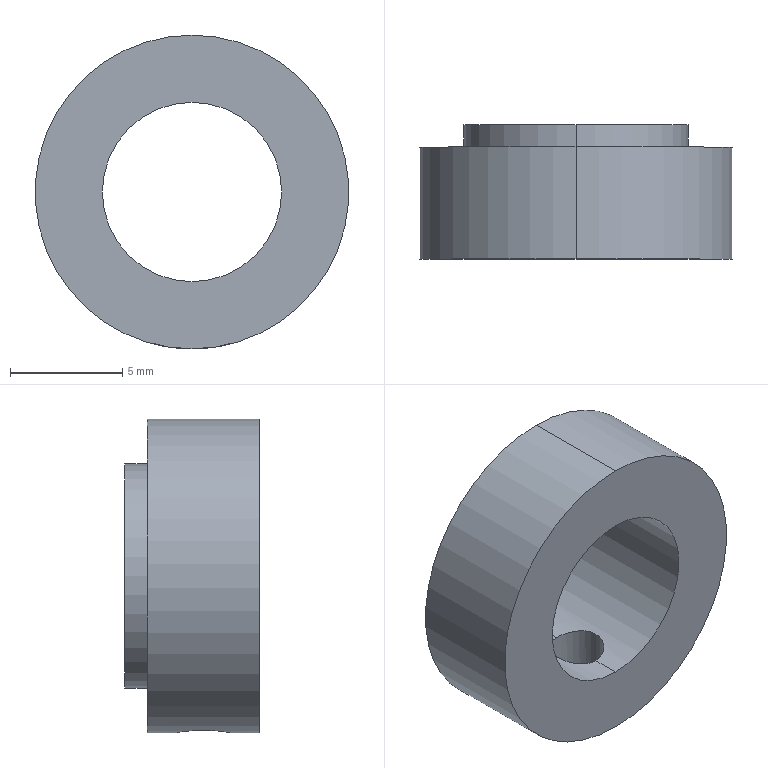Part | SolidWorks | features ICE 1, Revolution 1 | 1 solid | 11 faces | box 14 x 6 x 14 mm | volume 531.806 mm3 | cylinder 8 | plane 3 | commonest cylinder face diameters 2.5 x2 8 x2 10 x2 14 x2
STEP:
#1=CARTESIAN_POINT('',(0.,-0.3817,-7.));
#2=VERTEX_POINT('',#1);
#3=CARTESIAN_POINT('',(-1.25,0.8683,-6.887));
#4=VERTEX_POINT('',#3);
#5=CARTESIAN_POINT('',(0.,-0.3817,-7.));
#6=CARTESIAN_POINT('',(-0.1634,-0.3817,-7.));
#7=CARTESIAN_POINT('',(-0.3282,-0.3488,-6.994));
#8=CARTESIAN_POINT('',(-0.6292,-0.224,-6.973));
#9=CARTESIAN_POINT('',(-0.7683,-0.1311,-6.959));
#10=CARTESIAN_POINT('',(-0.9412,0.04171,-6.937));
#11=CARTESIAN_POINT('',(-0.994,0.1059,-6.929));
#12=CARTESIAN_POINT('',(-1.085,0.2414,-6.916));
#13=CARTESIAN_POINT('',(-1.123,0.3131,-6.909));
#14=CARTESIAN_POINT('',(-1.217,0.5406,-6.894));
#15=CARTESIAN_POINT('',(-1.25,0.7031,-6.887));
#16=CARTESIAN_POINT('',(-1.25,0.8683,-6.887));
#17=B_SPLINE_CURVE_WITH_KNOTS('',3,(#5,#6,#7,#8,#9,#10,#11,#12,#13,#14,#15,#16),.UNSPECIFIED.,.F.,.F.,(4,2,2,2,2,4),(0.003916,0.004405,0.004895,0.00514,0.005385,0.005874),.UNSPECIFIED.);
#18=EDGE_CURVE('',#2,#4,#17,.T.);
#19=ORIENTED_EDGE('',*,*,#18,.T.);
#20=CARTESIAN_POINT('',(-1.25,0.8683,-3.8));
#21=VERTEX_POINT('',#20);
#22=CARTESIAN_POINT('',(-1.25,0.8683,-10.));
#23=DIRECTION('',(0.,0.,1.));
#24=VECTOR('',#23,1000.);
#25=LINE('',#22,#24);
#26=EDGE_CURVE('',#4,#21,#25,.T.);
#27=ORIENTED_EDGE('',*,*,#26,.T.);
#28=CARTESIAN_POINT('',(0.,-0.3817,-4.));
#29=VERTEX_POINT('',#28);
#30=CARTESIAN_POINT('',(-1.25,0.8683,-3.8));
#31=CARTESIAN_POINT('',(-1.25,0.7862,-3.8));
#32=CARTESIAN_POINT('',(-1.242,0.7028,-3.802));
#33=CARTESIAN_POINT('',(-1.209,0.5421,-3.813));
#34=CARTESIAN_POINT('',(-1.186,0.4639,-3.82));
#35=CARTESIAN_POINT('',(-1.091,0.236,-3.849));
#36=CARTESIAN_POINT('',(-0.9987,0.09902,-3.875));
#37=CARTESIAN_POINT('',(-0.8257,-0.0737,-3.914));
#38=CARTESIAN_POINT('',(-0.7632,-0.125,-3.927));
#39=CARTESIAN_POINT('',(-0.6281,-0.2155,-3.951));
#40=CARTESIAN_POINT('',(-0.5549,-0.2548,-3.962));
#41=CARTESIAN_POINT('',(-0.329,-0.3486,-3.989));
#42=CARTESIAN_POINT('',(-0.1638,-0.3817,-4.));
#43=CARTESIAN_POINT('',(0.,-0.3817,-4.));
#44=B_SPLINE_CURVE_WITH_KNOTS('',3,(#30,#31,#32,#33,#34,#35,#36,#37,#38,#39,#40,#41,#42,#43),.UNSPECIFIED.,.F.,.F.,(4,2,2,2,2,2,4),(0.001967,0.002213,0.002458,0.00295,0.003196,0.003441,0.003933),.UNSPECIFIED.);
#45=EDGE_CURVE('',#21,#29,#44,.T.);
#46=ORIENTED_EDGE('',*,*,#45,.T.);
#47=CARTESIAN_POINT('',(1.25,0.8683,-3.8));
#48=VERTEX_POINT('',#47);
#49=CARTESIAN_POINT('',(0.,-0.3817,-4.));
#50=CARTESIAN_POINT('',(0.1638,-0.3817,-4.));
#51=CARTESIAN_POINT('',(0.3292,-0.3486,-3.989));
#52=CARTESIAN_POINT('',(0.6307,-0.2232,-3.953));
#53=CARTESIAN_POINT('',(0.7685,-0.131,-3.927));
#54=CARTESIAN_POINT('',(0.9992,0.09974,-3.875));
#55=CARTESIAN_POINT('',(1.091,0.236,-3.849));
#56=CARTESIAN_POINT('',(1.186,0.4643,-3.82));
#57=CARTESIAN_POINT('',(1.21,0.5424,-3.813));
#58=CARTESIAN_POINT('',(1.242,0.7027,-3.802));
#59=CARTESIAN_POINT('',(1.25,0.7859,-3.8));
#60=CARTESIAN_POINT('',(1.25,0.8683,-3.8));
#61=B_SPLINE_CURVE_WITH_KNOTS('',3,(#49,#50,#51,#52,#53,#54,#55,#56,#57,#58,#59,#60),.UNSPECIFIED.,.F.,.F.,(4,2,2,2,2,4),(0.003933,0.004424,0.004916,0.005407,0.005653,0.005899),.UNSPECIFIED.);
#62=EDGE_CURVE('',#29,#48,#61,.T.);
#63=ORIENTED_EDGE('',*,*,#62,.T.);
#64=CARTESIAN_POINT('',(1.25,0.8683,-6.887));
#65=VERTEX_POINT('',#64);
#66=CARTESIAN_POINT('',(1.25,0.8683,-10.));
#67=DIRECTION('',(0.,0.,1.));
#68=VECTOR('',#67,1000.);
#69=LINE('',#66,#68);
#70=EDGE_CURVE('',#65,#48,#69,.T.);
#71=ORIENTED_EDGE('',*,*,#70,.F.);
#72=CARTESIAN_POINT('',(1.25,0.8683,-6.887));
#73=CARTESIAN_POINT('',(1.25,0.7866,-6.887));
#74=CARTESIAN_POINT('',(1.242,0.7036,-6.889));
#75=CARTESIAN_POINT('',(1.21,0.5432,-6.895));
#76=CARTESIAN_POINT('',(1.186,0.4652,-6.899));
#77=CARTESIAN_POINT('',(1.092,0.238,-6.915));
#78=CARTESIAN_POINT('',(1.,0.1005,-6.929));
#79=CARTESIAN_POINT('',(0.7674,-0.1321,-6.959));
#80=CARTESIAN_POINT('',(0.6298,-0.2238,-6.973));
#81=CARTESIAN_POINT('',(0.3275,-0.3491,-6.994));
#82=CARTESIAN_POINT('',(0.1633,-0.3817,-7.));
#83=CARTESIAN_POINT('',(0.,-0.3817,-7.));
#84=B_SPLINE_CURVE_WITH_KNOTS('',3,(#72,#73,#74,#75,#76,#77,#78,#79,#80,#81,#82,#83),.UNSPECIFIED.,.F.,.F.,(4,2,2,2,2,4),(0.001958,0.002203,0.002448,0.002937,0.003427,0.003916),.UNSPECIFIED.);
#85=EDGE_CURVE('',#65,#2,#84,.T.);
#86=ORIENTED_EDGE('',*,*,#85,.T.);
#87=EDGE_LOOP('',(#19,#27,#46,#63,#71,#86));
#88=FACE_OUTER_BOUND('',#87,.T.);
#89=CARTESIAN_POINT('',(0.,0.8683,-10.));
#90=DIRECTION('',(0.,0.,1.));
#91=DIRECTION('',(1.,0.,0.));
#92=AXIS2_PLACEMENT_3D('',#89,#90,#91);
#93=CYLINDRICAL_SURFACE('',#92,1.25);
#94=ADVANCED_FACE('',(#88),#93,.F.);
#95=CARTESIAN_POINT('',(0.,3.368,-7.));
#96=VERTEX_POINT('',#95);
#97=CARTESIAN_POINT('',(0.,3.368,7.));
#98=VERTEX_POINT('',#97);
#99=CARTESIAN_POINT('',(0.,3.368,0.));
#100=DIRECTION('',(0.,-1.,0.));
#101=DIRECTION('',(0.,0.,-1.));
#102=AXIS2_PLACEMENT_3D('',#99,#100,#101);
#103=CIRCLE('',#102,7.);
#104=EDGE_CURVE('',#96,#98,#103,.T.);
#105=ORIENTED_EDGE('',*,*,#104,.T.);
#106=CARTESIAN_POINT('',(0.,-1.632,7.));
#107=VERTEX_POINT('',#106);
#108=CARTESIAN_POINT('',(0.,0.,7.));
#109=DIRECTION('',(0.,-1.,0.));
#110=VECTOR('',#109,1000.);
#111=LINE('',#108,#110);
#112=EDGE_CURVE('',#98,#107,#111,.T.);
#113=ORIENTED_EDGE('',*,*,#112,.T.);
#114=CARTESIAN_POINT('',(0.,-1.632,-7.));
#115=VERTEX_POINT('',#114);
#116=CARTESIAN_POINT('',(0.,-1.632,0.));
#117=DIRECTION('',(0.,-1.,0.));
#118=DIRECTION('',(0.,0.,-1.));
#119=AXIS2_PLACEMENT_3D('',#116,#117,#118);
#120=CIRCLE('',#119,7.);
#121=EDGE_CURVE('',#115,#107,#120,.T.);
#122=ORIENTED_EDGE('',*,*,#121,.F.);
#123=CARTESIAN_POINT('',(0.,0.,-7.));
#124=DIRECTION('',(0.,-1.,0.));
#125=VECTOR('',#124,1000.);
#126=LINE('',#123,#125);
#127=EDGE_CURVE('',#2,#115,#126,.T.);
#128=ORIENTED_EDGE('',*,*,#127,.F.);
#129=ORIENTED_EDGE('',*,*,#85,.F.);
#130=CARTESIAN_POINT('',(0.,2.118,-7.));
#131=VERTEX_POINT('',#130);
#132=CARTESIAN_POINT('',(0.,2.118,-7.));
#133=CARTESIAN_POINT('',(0.1656,2.118,-7.));
#134=CARTESIAN_POINT('',(0.328,2.086,-6.994));
#135=CARTESIAN_POINT('',(0.6307,1.96,-6.973));
#136=CARTESIAN_POINT('',(0.7692,1.867,-6.959));
#137=CARTESIAN_POINT('',(0.9993,1.637,-6.929));
#138=CARTESIAN_POINT('',(1.092,1.497,-6.915));
#139=CARTESIAN_POINT('',(1.217,1.197,-6.894));
#140=CARTESIAN_POINT('',(1.25,1.032,-6.887));
#141=CARTESIAN_POINT('',(1.25,0.8683,-6.887));
#142=B_SPLINE_CURVE_WITH_KNOTS('',3,(#132,#133,#134,#135,#136,#137,#138,#139,#140,#141),.UNSPECIFIED.,.F.,.F.,(4,2,2,2,4),(0.,0.0004896,0.0009792,0.001469,0.001958),.UNSPECIFIED.);
#143=EDGE_CURVE('',#131,#65,#142,.T.);
#144=ORIENTED_EDGE('',*,*,#143,.F.);
#145=CARTESIAN_POINT('',(0.,0.,-7.));
#146=DIRECTION('',(0.,-1.,0.));
#147=VECTOR('',#146,1000.);
#148=LINE('',#145,#147);
#149=EDGE_CURVE('',#96,#131,#148,.T.);
#150=ORIENTED_EDGE('',*,*,#149,.F.);
#151=EDGE_LOOP('',(#105,#113,#122,#128,#129,#144,#150));
#152=FACE_OUTER_BOUND('',#151,.T.);
#153=CARTESIAN_POINT('',(0.,0.,0.));
#154=DIRECTION('',(0.,-1.,0.));
#155=DIRECTION('',(0.,0.,-1.));
#156=AXIS2_PLACEMENT_3D('',#153,#154,#155);
#157=CYLINDRICAL_SURFACE('',#156,7.);
#158=ADVANCED_FACE('',(#152),#157,.T.);
#159=CARTESIAN_POINT('',(0.,4.368,-5.));
#160=VERTEX_POINT('',#159);
#161=CARTESIAN_POINT('',(0.,4.368,5.));
#162=VERTEX_POINT('',#161);
#163=CARTESIAN_POINT('',(0.,4.368,0.));
#164=DIRECTION('',(0.,-1.,0.));
#165=DIRECTION('',(0.,0.,-1.));
#166=AXIS2_PLACEMENT_3D('',#163,#164,#165);
#167=CIRCLE('',#166,5.);
#168=EDGE_CURVE('',#160,#162,#167,.T.);
#169=ORIENTED_EDGE('',*,*,#168,.T.);
#170=CARTESIAN_POINT('',(0.,3.368,5.));
#171=VERTEX_POINT('',#170);
#172=CARTESIAN_POINT('',(0.,0.,5.));
#173=DIRECTION('',(0.,-1.,0.));
#174=VECTOR('',#173,1000.);
#175=LINE('',#172,#174);
#176=EDGE_CURVE('',#162,#171,#175,.T.);
#177=ORIENTED_EDGE('',*,*,#176,.T.);
#178=CARTESIAN_POINT('',(0.,3.368,-5.));
#179=VERTEX_POINT('',#178);
#180=CARTESIAN_POINT('',(0.,3.368,0.));
#181=DIRECTION('',(0.,-1.,0.));
#182=DIRECTION('',(0.,0.,-1.));
#183=AXIS2_PLACEMENT_3D('',#180,#181,#182);
#184=CIRCLE('',#183,5.);
#185=EDGE_CURVE('',#179,#171,#184,.T.);
#186=ORIENTED_EDGE('',*,*,#185,.F.);
#187=CARTESIAN_POINT('',(0.,0.,-5.));
#188=DIRECTION('',(0.,-1.,0.));
#189=VECTOR('',#188,1000.);
#190=LINE('',#187,#189);
#191=EDGE_CURVE('',#160,#179,#190,.T.);
#192=ORIENTED_EDGE('',*,*,#191,.F.);
#193=EDGE_LOOP('',(#169,#177,#186,#192));
#194=FACE_OUTER_BOUND('',#193,.T.);
#195=CARTESIAN_POINT('',(0.,0.,0.));
#196=DIRECTION('',(0.,-1.,0.));
#197=DIRECTION('',(0.,0.,-1.));
#198=AXIS2_PLACEMENT_3D('',#195,#196,#197);
#199=CYLINDRICAL_SURFACE('',#198,5.);
#200=ADVANCED_FACE('',(#194),#199,.T.);
#201=CARTESIAN_POINT('',(0.,4.368,4.));
#202=VERTEX_POINT('',#201);
#203=CARTESIAN_POINT('',(0.,4.368,-4.));
#204=VERTEX_POINT('',#203);
#205=CARTESIAN_POINT('',(0.,4.368,0.));
#206=DIRECTION('',(0.,-1.,0.));
#207=DIRECTION('',(0.,0.,-1.));
#208=AXIS2_PLACEMENT_3D('',#205,#206,#207);
#209=CIRCLE('',#208,4.);
#210=EDGE_CURVE('',#202,#204,#209,.T.);
#211=ORIENTED_EDGE('',*,*,#210,.F.);
#212=CARTESIAN_POINT('',(0.,-1.632,4.));
#213=VERTEX_POINT('',#212);
#214=CARTESIAN_POINT('',(0.,0.,4.));
#215=DIRECTION('',(0.,-1.,0.));
#216=VECTOR('',#215,1000.);
#217=LINE('',#214,#216);
#218=EDGE_CURVE('',#202,#213,#217,.T.);
#219=ORIENTED_EDGE('',*,*,#218,.T.);
#220=CARTESIAN_POINT('',(0.,-1.632,-4.));
#221=VERTEX_POINT('',#220);
#222=CARTESIAN_POINT('',(0.,-1.632,0.));
#223=DIRECTION('',(0.,-1.,0.));
#224=DIRECTION('',(0.,0.,-1.));
#225=AXIS2_PLACEMENT_3D('',#222,#223,#224);
#226=CIRCLE('',#225,4.);
#227=EDGE_CURVE('',#213,#221,#226,.T.);
#228=ORIENTED_EDGE('',*,*,#227,.T.);
#229=CARTESIAN_POINT('',(0.,0.,-4.));
#230=DIRECTION('',(0.,-1.,0.));
#231=VECTOR('',#230,1000.);
#232=LINE('',#229,#231);
#233=EDGE_CURVE('',#29,#221,#232,.T.);
#234=ORIENTED_EDGE('',*,*,#233,.F.);
#235=ORIENTED_EDGE('',*,*,#45,.F.);
#236=CARTESIAN_POINT('',(0.,2.118,-4.));
#237=VERTEX_POINT('',#236);
#238=CARTESIAN_POINT('',(0.,2.118,-4.));
#239=CARTESIAN_POINT('',(-0.1664,2.118,-4.));
#240=CARTESIAN_POINT('',(-0.3295,2.085,-3.989));
#241=CARTESIAN_POINT('',(-0.6319,1.959,-3.953));
#242=CARTESIAN_POINT('',(-0.7699,1.866,-3.927));
#243=CARTESIAN_POINT('',(-0.9989,1.637,-3.875));
#244=CARTESIAN_POINT('',(-1.092,1.498,-3.849));
#245=CARTESIAN_POINT('',(-1.217,1.198,-3.811));
#246=CARTESIAN_POINT('',(-1.25,1.033,-3.8));
#247=CARTESIAN_POINT('',(-1.25,0.8683,-3.8));
#248=B_SPLINE_CURVE_WITH_KNOTS('',3,(#238,#239,#240,#241,#242,#243,#244,#245,#246,#247),.UNSPECIFIED.,.F.,.F.,(4,2,2,2,4),(0.,0.0004918,0.0009835,0.001475,0.001967),.UNSPECIFIED.);
#249=EDGE_CURVE('',#237,#21,#248,.T.);
#250=ORIENTED_EDGE('',*,*,#249,.F.);
#251=CARTESIAN_POINT('',(0.,0.,-4.));
#252=DIRECTION('',(0.,-1.,0.));
#253=VECTOR('',#252,1000.);
#254=LINE('',#251,#253);
#255=EDGE_CURVE('',#204,#237,#254,.T.);
#256=ORIENTED_EDGE('',*,*,#255,.F.);
#257=EDGE_LOOP('',(#211,#219,#228,#234,#235,#250,#256));
#258=FACE_OUTER_BOUND('',#257,.T.);
#259=CARTESIAN_POINT('',(0.,0.,0.));
#260=DIRECTION('',(0.,-1.,0.));
#261=DIRECTION('',(0.,0.,-1.));
#262=AXIS2_PLACEMENT_3D('',#259,#260,#261);
#263=CYLINDRICAL_SURFACE('',#262,4.);
#264=ADVANCED_FACE('',(#258),#263,.F.);
#265=ORIENTED_EDGE('',*,*,#218,.F.);
#266=CARTESIAN_POINT('',(0.,4.368,0.));
#267=DIRECTION('',(0.,-1.,0.));
#268=DIRECTION('',(0.,0.,-1.));
#269=AXIS2_PLACEMENT_3D('',#266,#267,#268);
#270=CIRCLE('',#269,4.);
#271=EDGE_CURVE('',#204,#202,#270,.T.);
#272=ORIENTED_EDGE('',*,*,#271,.F.);
#273=ORIENTED_EDGE('',*,*,#255,.T.);
#274=CARTESIAN_POINT('',(1.25,0.8683,-3.8));
#275=CARTESIAN_POINT('',(1.25,1.033,-3.8));
#276=CARTESIAN_POINT('',(1.217,1.198,-3.811));
#277=CARTESIAN_POINT('',(1.092,1.499,-3.849));
#278=CARTESIAN_POINT('',(0.9987,1.637,-3.875));
#279=CARTESIAN_POINT('',(0.7696,1.866,-3.927));
#280=CARTESIAN_POINT('',(0.6317,1.959,-3.953));
#281=CARTESIAN_POINT('',(0.3299,2.085,-3.989));
#282=CARTESIAN_POINT('',(0.1663,2.118,-4.));
#283=CARTESIAN_POINT('',(0.,2.118,-4.));
#284=B_SPLINE_CURVE_WITH_KNOTS('',3,(#274,#275,#276,#277,#278,#279,#280,#281,#282,#283),.UNSPECIFIED.,.F.,.F.,(4,2,2,2,4),(0.005899,0.00639,0.006882,0.007373,0.007865),.UNSPECIFIED.);
#285=EDGE_CURVE('',#48,#237,#284,.T.);
#286=ORIENTED_EDGE('',*,*,#285,.F.);
#287=ORIENTED_EDGE('',*,*,#62,.F.);
#288=ORIENTED_EDGE('',*,*,#233,.T.);
#289=CARTESIAN_POINT('',(0.,-1.632,0.));
#290=DIRECTION('',(0.,-1.,0.));
#291=DIRECTION('',(0.,0.,-1.));
#292=AXIS2_PLACEMENT_3D('',#289,#290,#291);
#293=CIRCLE('',#292,4.);
#294=EDGE_CURVE('',#221,#213,#293,.T.);
#295=ORIENTED_EDGE('',*,*,#294,.T.);
#296=EDGE_LOOP('',(#265,#272,#273,#286,#287,#288,#295));
#297=FACE_OUTER_BOUND('',#296,.T.);
#298=CARTESIAN_POINT('',(0.,0.,0.));
#299=DIRECTION('',(0.,-1.,0.));
#300=DIRECTION('',(0.,0.,-1.));
#301=AXIS2_PLACEMENT_3D('',#298,#299,#300);
#302=CYLINDRICAL_SURFACE('',#301,4.);
#303=ADVANCED_FACE('',(#297),#302,.F.);
#304=ORIENTED_EDGE('',*,*,#271,.T.);
#305=ORIENTED_EDGE('',*,*,#210,.T.);
#306=EDGE_LOOP('',(#304,#305));
#307=FACE_BOUND('',#306,.T.);
#308=ORIENTED_EDGE('',*,*,#168,.F.);
#309=CARTESIAN_POINT('',(0.,4.368,0.));
#310=DIRECTION('',(0.,-1.,0.));
#311=DIRECTION('',(0.,0.,-1.));
#312=AXIS2_PLACEMENT_3D('',#309,#310,#311);
#313=CIRCLE('',#312,5.);
#314=EDGE_CURVE('',#162,#160,#313,.T.);
#315=ORIENTED_EDGE('',*,*,#314,.F.);
#316=EDGE_LOOP('',(#308,#315));
#317=FACE_OUTER_BOUND('',#316,.T.);
#318=CARTESIAN_POINT('',(4.,4.368,0.));
#319=DIRECTION('',(0.,1.,0.));
#320=DIRECTION('',(0.,0.,1.));
#321=AXIS2_PLACEMENT_3D('',#318,#319,#320);
#322=PLANE('',#321);
#323=ADVANCED_FACE('',(#307,#317),#322,.T.);
#324=ORIENTED_EDGE('',*,*,#176,.F.);
#325=ORIENTED_EDGE('',*,*,#314,.T.);
#326=ORIENTED_EDGE('',*,*,#191,.T.);
#327=CARTESIAN_POINT('',(0.,3.368,0.));
#328=DIRECTION('',(0.,-1.,0.));
#329=DIRECTION('',(0.,0.,-1.));
#330=AXIS2_PLACEMENT_3D('',#327,#328,#329);
#331=CIRCLE('',#330,5.);
#332=EDGE_CURVE('',#171,#179,#331,.T.);
#333=ORIENTED_EDGE('',*,*,#332,.F.);
#334=EDGE_LOOP('',(#324,#325,#326,#333));
#335=FACE_OUTER_BOUND('',#334,.T.);
#336=CARTESIAN_POINT('',(0.,0.,0.));
#337=DIRECTION('',(0.,-1.,0.));
#338=DIRECTION('',(0.,0.,-1.));
#339=AXIS2_PLACEMENT_3D('',#336,#337,#338);
#340=CYLINDRICAL_SURFACE('',#339,5.);
#341=ADVANCED_FACE('',(#335),#340,.T.);
#342=ORIENTED_EDGE('',*,*,#185,.T.);
#343=ORIENTED_EDGE('',*,*,#332,.T.);
#344=EDGE_LOOP('',(#342,#343));
#345=FACE_BOUND('',#344,.T.);
#346=ORIENTED_EDGE('',*,*,#104,.F.);
#347=CARTESIAN_POINT('',(0.,3.368,0.));
#348=DIRECTION('',(0.,-1.,0.));
#349=DIRECTION('',(0.,0.,-1.));
#350=AXIS2_PLACEMENT_3D('',#347,#348,#349);
#351=CIRCLE('',#350,7.);
#352=EDGE_CURVE('',#98,#96,#351,.T.);
#353=ORIENTED_EDGE('',*,*,#352,.F.);
#354=EDGE_LOOP('',(#346,#353));
#355=FACE_OUTER_BOUND('',#354,.T.);
#356=CARTESIAN_POINT('',(5.,3.368,0.));
#357=DIRECTION('',(0.,1.,0.));
#358=DIRECTION('',(0.,0.,1.));
#359=AXIS2_PLACEMENT_3D('',#356,#357,#358);
#360=PLANE('',#359);
#361=ADVANCED_FACE('',(#345,#355),#360,.T.);
#362=ORIENTED_EDGE('',*,*,#112,.F.);
#363=ORIENTED_EDGE('',*,*,#352,.T.);
#364=ORIENTED_EDGE('',*,*,#149,.T.);
#365=CARTESIAN_POINT('',(-1.25,0.8683,-6.887));
#366=CARTESIAN_POINT('',(-1.25,1.033,-6.887));
#367=CARTESIAN_POINT('',(-1.217,1.196,-6.894));
#368=CARTESIAN_POINT('',(-1.092,1.498,-6.915));
#369=CARTESIAN_POINT('',(-0.9991,1.637,-6.929));
#370=CARTESIAN_POINT('',(-0.7693,1.867,-6.959));
#371=CARTESIAN_POINT('',(-0.6302,1.96,-6.973));
#372=CARTESIAN_POINT('',(-0.3297,2.085,-6.994));
#373=CARTESIAN_POINT('',(-0.1654,2.118,-7.));
#374=CARTESIAN_POINT('',(0.,2.118,-7.));
#375=B_SPLINE_CURVE_WITH_KNOTS('',3,(#365,#366,#367,#368,#369,#370,#371,#372,#373,#374),.UNSPECIFIED.,.F.,.F.,(4,2,2,2,4),(0.005874,0.006363,0.006852,0.007342,0.007831),.UNSPECIFIED.);
#376=EDGE_CURVE('',#4,#131,#375,.T.);
#377=ORIENTED_EDGE('',*,*,#376,.F.);
#378=ORIENTED_EDGE('',*,*,#18,.F.);
#379=ORIENTED_EDGE('',*,*,#127,.T.);
#380=CARTESIAN_POINT('',(0.,-1.632,0.));
#381=DIRECTION('',(0.,-1.,0.));
#382=DIRECTION('',(0.,0.,-1.));
#383=AXIS2_PLACEMENT_3D('',#380,#381,#382);
#384=CIRCLE('',#383,7.);
#385=EDGE_CURVE('',#107,#115,#384,.T.);
#386=ORIENTED_EDGE('',*,*,#385,.F.);
#387=EDGE_LOOP('',(#362,#363,#364,#377,#378,#379,#386));
#388=FACE_OUTER_BOUND('',#387,.T.);
#389=CARTESIAN_POINT('',(0.,0.,0.));
#390=DIRECTION('',(0.,-1.,0.));
#391=DIRECTION('',(0.,0.,-1.));
#392=AXIS2_PLACEMENT_3D('',#389,#390,#391);
#393=CYLINDRICAL_SURFACE('',#392,7.);
#394=ADVANCED_FACE('',(#388),#393,.T.);
#395=ORIENTED_EDGE('',*,*,#121,.T.);
#396=ORIENTED_EDGE('',*,*,#385,.T.);
#397=EDGE_LOOP('',(#395,#396));
#398=FACE_OUTER_BOUND('',#397,.T.);
#399=ORIENTED_EDGE('',*,*,#294,.F.);
#400=ORIENTED_EDGE('',*,*,#227,.F.);
#401=EDGE_LOOP('',(#399,#400));
#402=FACE_BOUND('',#401,.T.);
#403=CARTESIAN_POINT('',(7.,-1.632,0.));
#404=DIRECTION('',(0.,-1.,0.));
#405=DIRECTION('',(0.,0.,-1.));
#406=AXIS2_PLACEMENT_3D('',#403,#404,#405);
#407=PLANE('',#406);
#408=ADVANCED_FACE('',(#398,#402),#407,.T.);
#409=ORIENTED_EDGE('',*,*,#26,.F.);
#410=ORIENTED_EDGE('',*,*,#376,.T.);
#411=ORIENTED_EDGE('',*,*,#143,.T.);
#412=ORIENTED_EDGE('',*,*,#70,.T.);
#413=ORIENTED_EDGE('',*,*,#285,.T.);
#414=ORIENTED_EDGE('',*,*,#249,.T.);
#415=EDGE_LOOP('',(#409,#410,#411,#412,#413,#414));
#416=FACE_OUTER_BOUND('',#415,.T.);
#417=CARTESIAN_POINT('',(0.,0.8683,-10.));
#418=DIRECTION('',(0.,0.,1.));
#419=DIRECTION('',(1.,0.,0.));
#420=AXIS2_PLACEMENT_3D('',#417,#418,#419);
#421=CYLINDRICAL_SURFACE('',#420,1.25);
#422=ADVANCED_FACE('',(#416),#421,.F.);
#423=CLOSED_SHELL('',(#94,#158,#200,#264,#303,#323,#341,#361,#394,#408,#422));
#424=MANIFOLD_SOLID_BREP('',#423);
#425=CARTESIAN_POINT('',(0.,0.,0.));
#426=DIRECTION('',(0.,0.,1.));
#427=DIRECTION('',(1.,0.,0.));
#428=AXIS2_PLACEMENT_3D('',#425,#426,#427);
#429=(LENGTH_UNIT()NAMED_UNIT(*)SI_UNIT(.MILLI.,.METRE.));
#430=UNCERTAINTY_MEASURE_WITH_UNIT(LENGTH_MEASURE(0.00001),#429,'','');
#431=(NAMED_UNIT(*)PLANE_ANGLE_UNIT()SI_UNIT($,.RADIAN.));
#432=(NAMED_UNIT(*)SI_UNIT($,.STERADIAN.)SOLID_ANGLE_UNIT());
#433=(GEOMETRIC_REPRESENTATION_CONTEXT(3)GLOBAL_UNCERTAINTY_ASSIGNED_CONTEXT((#430))GLOBAL_UNIT_ASSIGNED_CONTEXT((#429,#431,#432))REPRESENTATION_CONTEXT('',''));
#434=ADVANCED_BREP_SHAPE_REPRESENTATION('',(#424,#428),#433);